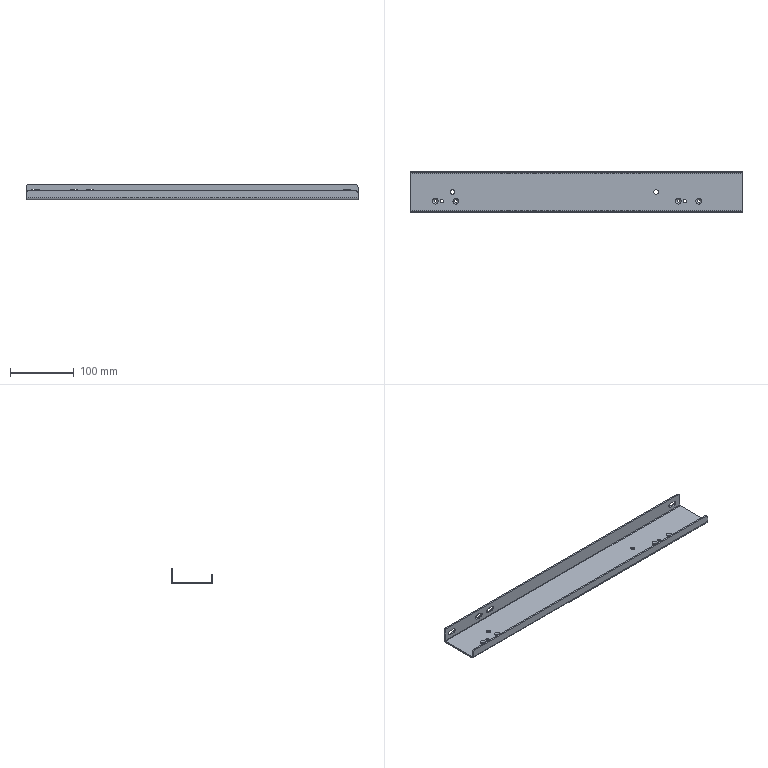Part | SolidWorks | features MirrorStock 1 | 1 solid | 76 faces | box 522 x 65 x 25 mm | volume 126606 mm3 | cylinder 38 | plane 30 | cone 8 | commonest cylinder face diameters 7 x12 4.5 x8 8 x6 5.5 x4 10 x4 1.473 x2